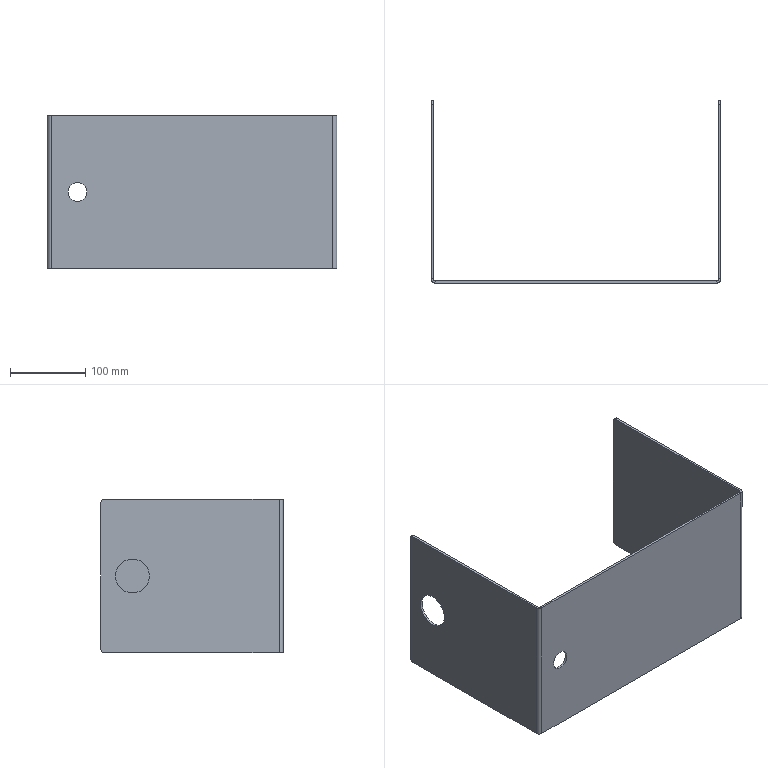Part | SolidWorks | features ICE 2, Fillet 1, FlatPattern 1, SMBaseFlange 1, SheetMetal 1, UnFold 1 | 1 solid | 30 faces | box 384 x 242 x 204 mm | volume 519134 mm3 | plane 18 | cylinder 12 | commonest cylinder face diameters 10 x4 5 x2 11 x2 25 x2 45 x2
STEP:
#1=CARTESIAN_POINT('',(-152.,0.,-12.5));
#2=VERTEX_POINT('',#1);
#3=CARTESIAN_POINT('',(-152.,0.,12.5));
#4=VERTEX_POINT('',#3);
#5=CARTESIAN_POINT('',(-152.,0.,0.));
#6=DIRECTION('',(0.,1.,0.));
#7=DIRECTION('',(0.,0.,1.));
#8=AXIS2_PLACEMENT_3D('',#5,#6,#7);
#9=CIRCLE('',#8,12.5);
#10=EDGE_CURVE('',#2,#4,#9,.T.);
#11=ORIENTED_EDGE('',*,*,#10,.F.);
#12=CARTESIAN_POINT('',(-152.,3.,-12.5));
#13=VERTEX_POINT('',#12);
#14=CARTESIAN_POINT('',(-152.,0.,-12.5));
#15=DIRECTION('',(0.,1.,0.));
#16=VECTOR('',#15,1000.);
#17=LINE('',#14,#16);
#18=EDGE_CURVE('',#2,#13,#17,.T.);
#19=ORIENTED_EDGE('',*,*,#18,.T.);
#20=CARTESIAN_POINT('',(-152.,3.,12.5));
#21=VERTEX_POINT('',#20);
#22=CARTESIAN_POINT('',(-152.,3.,0.));
#23=DIRECTION('',(0.,1.,0.));
#24=DIRECTION('',(0.,0.,1.));
#25=AXIS2_PLACEMENT_3D('',#22,#23,#24);
#26=CIRCLE('',#25,12.5);
#27=EDGE_CURVE('',#13,#21,#26,.T.);
#28=ORIENTED_EDGE('',*,*,#27,.T.);
#29=CARTESIAN_POINT('',(-152.,0.,12.5));
#30=DIRECTION('',(0.,1.,0.));
#31=VECTOR('',#30,1000.);
#32=LINE('',#29,#31);
#33=EDGE_CURVE('',#4,#21,#32,.T.);
#34=ORIENTED_EDGE('',*,*,#33,.F.);
#35=EDGE_LOOP('',(#11,#19,#28,#34));
#36=FACE_OUTER_BOUND('',#35,.T.);
#37=CARTESIAN_POINT('',(-152.,0.,0.));
#38=DIRECTION('',(0.,1.,0.));
#39=DIRECTION('',(0.,0.,1.));
#40=AXIS2_PLACEMENT_3D('',#37,#38,#39);
#41=CYLINDRICAL_SURFACE('',#40,12.5);
#42=ADVANCED_FACE('',(#36),#41,.F.);
#43=CARTESIAN_POINT('',(-189.,200.,-22.5));
#44=VERTEX_POINT('',#43);
#45=CARTESIAN_POINT('',(-189.,200.,22.5));
#46=VERTEX_POINT('',#45);
#47=CARTESIAN_POINT('',(-189.,200.,0.));
#48=DIRECTION('',(-1.,0.,0.));
#49=DIRECTION('',(0.,0.,1.));
#50=AXIS2_PLACEMENT_3D('',#47,#48,#49);
#51=CIRCLE('',#50,22.5);
#52=EDGE_CURVE('',#44,#46,#51,.T.);
#53=ORIENTED_EDGE('',*,*,#52,.F.);
#54=CARTESIAN_POINT('',(-192.,200.,-22.5));
#55=VERTEX_POINT('',#54);
#56=CARTESIAN_POINT('',(-189.,200.,-22.5));
#57=DIRECTION('',(-1.,0.,0.));
#58=VECTOR('',#57,1000.);
#59=LINE('',#56,#58);
#60=EDGE_CURVE('',#44,#55,#59,.T.);
#61=ORIENTED_EDGE('',*,*,#60,.T.);
#62=CARTESIAN_POINT('',(-192.,200.,22.5));
#63=VERTEX_POINT('',#62);
#64=CARTESIAN_POINT('',(-192.,200.,0.));
#65=DIRECTION('',(-1.,0.,0.));
#66=DIRECTION('',(0.,0.,1.));
#67=AXIS2_PLACEMENT_3D('',#64,#65,#66);
#68=CIRCLE('',#67,22.5);
#69=EDGE_CURVE('',#55,#63,#68,.T.);
#70=ORIENTED_EDGE('',*,*,#69,.T.);
#71=CARTESIAN_POINT('',(-189.,200.,22.5));
#72=DIRECTION('',(-1.,0.,0.));
#73=VECTOR('',#72,1000.);
#74=LINE('',#71,#73);
#75=EDGE_CURVE('',#46,#63,#74,.T.);
#76=ORIENTED_EDGE('',*,*,#75,.F.);
#77=EDGE_LOOP('',(#53,#61,#70,#76));
#78=FACE_OUTER_BOUND('',#77,.T.);
#79=CARTESIAN_POINT('',(-189.,200.,0.));
#80=DIRECTION('',(-1.,0.,0.));
#81=DIRECTION('',(0.,0.,1.));
#82=AXIS2_PLACEMENT_3D('',#79,#80,#81);
#83=CYLINDRICAL_SURFACE('',#82,22.5);
#84=ADVANCED_FACE('',(#78),#83,.F.);
#85=CARTESIAN_POINT('',(186.5,0.,102.));
#86=VERTEX_POINT('',#85);
#87=CARTESIAN_POINT('',(186.5,3.,102.));
#88=VERTEX_POINT('',#87);
#89=CARTESIAN_POINT('',(186.5,0.,102.));
#90=DIRECTION('',(0.,1.,0.));
#91=VECTOR('',#90,1000.);
#92=LINE('',#89,#91);
#93=EDGE_CURVE('',#86,#88,#92,.T.);
#94=ORIENTED_EDGE('',*,*,#93,.F.);
#95=CARTESIAN_POINT('',(192.,5.5,102.));
#96=VERTEX_POINT('',#95);
#97=CARTESIAN_POINT('',(186.5,5.5,102.));
#98=DIRECTION('',(0.,0.,-1.));
#99=DIRECTION('',(1.,0.,0.));
#100=AXIS2_PLACEMENT_3D('',#97,#98,#99);
#101=CIRCLE('',#100,5.5);
#102=EDGE_CURVE('',#96,#86,#101,.T.);
#103=ORIENTED_EDGE('',*,*,#102,.F.);
#104=CARTESIAN_POINT('',(189.,5.5,102.));
#105=VERTEX_POINT('',#104);
#106=CARTESIAN_POINT('',(189.,5.5,102.));
#107=DIRECTION('',(1.,0.,0.));
#108=VECTOR('',#107,1000.);
#109=LINE('',#106,#108);
#110=EDGE_CURVE('',#105,#96,#109,.T.);
#111=ORIENTED_EDGE('',*,*,#110,.F.);
#112=CARTESIAN_POINT('',(186.5,5.5,102.));
#113=DIRECTION('',(0.,0.,-1.));
#114=DIRECTION('',(1.,0.,0.));
#115=AXIS2_PLACEMENT_3D('',#112,#113,#114);
#116=CIRCLE('',#115,2.5);
#117=EDGE_CURVE('',#105,#88,#116,.T.);
#118=ORIENTED_EDGE('',*,*,#117,.T.);
#119=EDGE_LOOP('',(#94,#103,#111,#118));
#120=FACE_OUTER_BOUND('',#119,.T.);
#121=CARTESIAN_POINT('',(186.5,0.,102.));
#122=DIRECTION('',(0.,0.,1.));
#123=DIRECTION('',(1.,0.,0.));
#124=AXIS2_PLACEMENT_3D('',#121,#122,#123);
#125=PLANE('',#124);
#126=ADVANCED_FACE('',(#120),#125,.T.);
#127=CARTESIAN_POINT('',(-186.5,0.,102.));
#128=VERTEX_POINT('',#127);
#129=CARTESIAN_POINT('',(-192.,0.,102.));
#130=DIRECTION('',(-1.,0.,0.));
#131=VECTOR('',#130,1000.);
#132=LINE('',#129,#131);
#133=EDGE_CURVE('',#86,#128,#132,.T.);
#134=ORIENTED_EDGE('',*,*,#133,.F.);
#135=ORIENTED_EDGE('',*,*,#93,.T.);
#136=CARTESIAN_POINT('',(-186.5,3.,102.));
#137=VERTEX_POINT('',#136);
#138=CARTESIAN_POINT('',(-192.,3.,102.));
#139=DIRECTION('',(-1.,0.,0.));
#140=VECTOR('',#139,1000.);
#141=LINE('',#138,#140);
#142=EDGE_CURVE('',#88,#137,#141,.T.);
#143=ORIENTED_EDGE('',*,*,#142,.T.);
#144=CARTESIAN_POINT('',(-186.5,3.,102.));
#145=DIRECTION('',(0.,-1.,0.));
#146=VECTOR('',#145,1000.);
#147=LINE('',#144,#146);
#148=EDGE_CURVE('',#137,#128,#147,.T.);
#149=ORIENTED_EDGE('',*,*,#148,.T.);
#150=EDGE_LOOP('',(#134,#135,#143,#149));
#151=FACE_OUTER_BOUND('',#150,.T.);
#152=CARTESIAN_POINT('',(189.,5.5,102.));
#153=DIRECTION('',(0.,0.,1.));
#154=DIRECTION('',(1.,0.,0.));
#155=AXIS2_PLACEMENT_3D('',#152,#153,#154);
#156=PLANE('',#155);
#157=ADVANCED_FACE('',(#151),#156,.T.);
#158=CARTESIAN_POINT('',(192.,5.5,-102.));
#159=VERTEX_POINT('',#158);
#160=CARTESIAN_POINT('',(189.,5.5,-102.));
#161=VERTEX_POINT('',#160);
#162=CARTESIAN_POINT('',(192.,5.5,-102.));
#163=DIRECTION('',(-1.,0.,0.));
#164=VECTOR('',#163,1000.);
#165=LINE('',#162,#164);
#166=EDGE_CURVE('',#159,#161,#165,.T.);
#167=ORIENTED_EDGE('',*,*,#166,.F.);
#168=CARTESIAN_POINT('',(186.5,0.,-102.));
#169=VERTEX_POINT('',#168);
#170=CARTESIAN_POINT('',(186.5,5.5,-102.));
#171=DIRECTION('',(0.,0.,-1.));
#172=DIRECTION('',(1.,0.,0.));
#173=AXIS2_PLACEMENT_3D('',#170,#171,#172);
#174=CIRCLE('',#173,5.5);
#175=EDGE_CURVE('',#159,#169,#174,.T.);
#176=ORIENTED_EDGE('',*,*,#175,.T.);
#177=CARTESIAN_POINT('',(186.5,3.,-102.));
#178=VERTEX_POINT('',#177);
#179=CARTESIAN_POINT('',(186.5,3.,-102.));
#180=DIRECTION('',(0.,-1.,0.));
#181=VECTOR('',#180,1000.);
#182=LINE('',#179,#181);
#183=EDGE_CURVE('',#178,#169,#182,.T.);
#184=ORIENTED_EDGE('',*,*,#183,.F.);
#185=CARTESIAN_POINT('',(186.5,5.5,-102.));
#186=DIRECTION('',(0.,0.,-1.));
#187=DIRECTION('',(1.,0.,0.));
#188=AXIS2_PLACEMENT_3D('',#185,#186,#187);
#189=CIRCLE('',#188,2.5);
#190=EDGE_CURVE('',#161,#178,#189,.T.);
#191=ORIENTED_EDGE('',*,*,#190,.F.);
#192=EDGE_LOOP('',(#167,#176,#184,#191));
#193=FACE_OUTER_BOUND('',#192,.T.);
#194=CARTESIAN_POINT('',(192.,5.5,-102.));
#195=DIRECTION('',(0.,0.,-1.));
#196=DIRECTION('',(-1.,0.,0.));
#197=AXIS2_PLACEMENT_3D('',#194,#195,#196);
#198=PLANE('',#197);
#199=ADVANCED_FACE('',(#193),#198,.T.);
#200=CARTESIAN_POINT('',(189.,237.,-102.));
#201=VERTEX_POINT('',#200);
#202=CARTESIAN_POINT('',(189.,0.,-102.));
#203=DIRECTION('',(0.,-1.,0.));
#204=VECTOR('',#203,1000.);
#205=LINE('',#202,#204);
#206=EDGE_CURVE('',#201,#161,#205,.T.);
#207=ORIENTED_EDGE('',*,*,#206,.F.);
#208=CARTESIAN_POINT('',(192.,237.,-102.));
#209=VERTEX_POINT('',#208);
#210=CARTESIAN_POINT('',(186.5,237.,-102.));
#211=DIRECTION('',(1.,0.,0.));
#212=VECTOR('',#211,1000.);
#213=LINE('',#210,#212);
#214=EDGE_CURVE('',#201,#209,#213,.T.);
#215=ORIENTED_EDGE('',*,*,#214,.T.);
#216=CARTESIAN_POINT('',(192.,0.,-102.));
#217=DIRECTION('',(0.,-1.,0.));
#218=VECTOR('',#217,1000.);
#219=LINE('',#216,#218);
#220=EDGE_CURVE('',#209,#159,#219,.T.);
#221=ORIENTED_EDGE('',*,*,#220,.T.);
#222=ORIENTED_EDGE('',*,*,#166,.T.);
#223=EDGE_LOOP('',(#207,#215,#221,#222));
#224=FACE_OUTER_BOUND('',#223,.T.);
#225=CARTESIAN_POINT('',(186.5,3.,-102.));
#226=DIRECTION('',(0.,0.,-1.));
#227=DIRECTION('',(-1.,0.,0.));
#228=AXIS2_PLACEMENT_3D('',#225,#226,#227);
#229=PLANE('',#228);
#230=ADVANCED_FACE('',(#224),#229,.T.);
#231=CARTESIAN_POINT('',(-192.,5.5,102.));
#232=VERTEX_POINT('',#231);
#233=CARTESIAN_POINT('',(-189.,5.5,102.));
#234=VERTEX_POINT('',#233);
#235=CARTESIAN_POINT('',(-192.,5.5,102.));
#236=DIRECTION('',(1.,0.,0.));
#237=VECTOR('',#236,1000.);
#238=LINE('',#235,#237);
#239=EDGE_CURVE('',#232,#234,#238,.T.);
#240=ORIENTED_EDGE('',*,*,#239,.F.);
#241=CARTESIAN_POINT('',(-186.5,5.5,102.));
#242=DIRECTION('',(0.,0.,-1.));
#243=DIRECTION('',(1.,0.,0.));
#244=AXIS2_PLACEMENT_3D('',#241,#242,#243);
#245=CIRCLE('',#244,5.5);
#246=EDGE_CURVE('',#128,#232,#245,.T.);
#247=ORIENTED_EDGE('',*,*,#246,.F.);
#248=ORIENTED_EDGE('',*,*,#148,.F.);
#249=CARTESIAN_POINT('',(-186.5,5.5,102.));
#250=DIRECTION('',(0.,0.,-1.));
#251=DIRECTION('',(1.,0.,0.));
#252=AXIS2_PLACEMENT_3D('',#249,#250,#251);
#253=CIRCLE('',#252,2.5);
#254=EDGE_CURVE('',#137,#234,#253,.T.);
#255=ORIENTED_EDGE('',*,*,#254,.T.);
#256=EDGE_LOOP('',(#240,#247,#248,#255));
#257=FACE_OUTER_BOUND('',#256,.T.);
#258=CARTESIAN_POINT('',(-192.,5.5,102.));
#259=DIRECTION('',(0.,0.,1.));
#260=DIRECTION('',(1.,0.,0.));
#261=AXIS2_PLACEMENT_3D('',#258,#259,#260);
#262=PLANE('',#261);
#263=ADVANCED_FACE('',(#257),#262,.T.);
#264=CARTESIAN_POINT('',(-189.,237.,102.));
#265=VERTEX_POINT('',#264);
#266=CARTESIAN_POINT('',(-189.,0.,102.));
#267=DIRECTION('',(0.,1.,0.));
#268=VECTOR('',#267,1000.);
#269=LINE('',#266,#268);
#270=EDGE_CURVE('',#234,#265,#269,.T.);
#271=ORIENTED_EDGE('',*,*,#270,.T.);
#272=CARTESIAN_POINT('',(-192.,237.,102.));
#273=VERTEX_POINT('',#272);
#274=CARTESIAN_POINT('',(-186.5,237.,102.));
#275=DIRECTION('',(-1.,0.,0.));
#276=VECTOR('',#275,1000.);
#277=LINE('',#274,#276);
#278=EDGE_CURVE('',#265,#273,#277,.T.);
#279=ORIENTED_EDGE('',*,*,#278,.T.);
#280=CARTESIAN_POINT('',(-192.,0.,102.));
#281=DIRECTION('',(0.,1.,0.));
#282=VECTOR('',#281,1000.);
#283=LINE('',#280,#282);
#284=EDGE_CURVE('',#232,#273,#283,.T.);
#285=ORIENTED_EDGE('',*,*,#284,.F.);
#286=ORIENTED_EDGE('',*,*,#239,.T.);
#287=EDGE_LOOP('',(#271,#279,#285,#286));
#288=FACE_OUTER_BOUND('',#287,.T.);
#289=CARTESIAN_POINT('',(-186.5,3.,102.));
#290=DIRECTION('',(0.,0.,1.));
#291=DIRECTION('',(1.,0.,0.));
#292=AXIS2_PLACEMENT_3D('',#289,#290,#291);
#293=PLANE('',#292);
#294=ADVANCED_FACE('',(#288),#293,.T.);
#295=CARTESIAN_POINT('',(-186.5,0.,-102.));
#296=VERTEX_POINT('',#295);
#297=CARTESIAN_POINT('',(-186.5,3.,-102.));
#298=VERTEX_POINT('',#297);
#299=CARTESIAN_POINT('',(-186.5,0.,-102.));
#300=DIRECTION('',(0.,1.,0.));
#301=VECTOR('',#300,1000.);
#302=LINE('',#299,#301);
#303=EDGE_CURVE('',#296,#298,#302,.T.);
#304=ORIENTED_EDGE('',*,*,#303,.F.);
#305=CARTESIAN_POINT('',(-192.,5.5,-102.));
#306=VERTEX_POINT('',#305);
#307=CARTESIAN_POINT('',(-186.5,5.5,-102.));
#308=DIRECTION('',(0.,0.,-1.));
#309=DIRECTION('',(1.,0.,0.));
#310=AXIS2_PLACEMENT_3D('',#307,#308,#309);
#311=CIRCLE('',#310,5.5);
#312=EDGE_CURVE('',#296,#306,#311,.T.);
#313=ORIENTED_EDGE('',*,*,#312,.T.);
#314=CARTESIAN_POINT('',(-189.,5.5,-102.));
#315=VERTEX_POINT('',#314);
#316=CARTESIAN_POINT('',(-189.,5.5,-102.));
#317=DIRECTION('',(-1.,0.,0.));
#318=VECTOR('',#317,1000.);
#319=LINE('',#316,#318);
#320=EDGE_CURVE('',#315,#306,#319,.T.);
#321=ORIENTED_EDGE('',*,*,#320,.F.);
#322=CARTESIAN_POINT('',(-186.5,5.5,-102.));
#323=DIRECTION('',(0.,0.,-1.));
#324=DIRECTION('',(1.,0.,0.));
#325=AXIS2_PLACEMENT_3D('',#322,#323,#324);
#326=CIRCLE('',#325,2.5);
#327=EDGE_CURVE('',#298,#315,#326,.T.);
#328=ORIENTED_EDGE('',*,*,#327,.F.);
#329=EDGE_LOOP('',(#304,#313,#321,#328));
#330=FACE_OUTER_BOUND('',#329,.T.);
#331=CARTESIAN_POINT('',(-186.5,0.,-102.));
#332=DIRECTION('',(0.,0.,-1.));
#333=DIRECTION('',(-1.,0.,0.));
#334=AXIS2_PLACEMENT_3D('',#331,#332,#333);
#335=PLANE('',#334);
#336=ADVANCED_FACE('',(#330),#335,.T.);
#337=CARTESIAN_POINT('',(-192.,0.,-102.));
#338=DIRECTION('',(-1.,0.,0.));
#339=VECTOR('',#338,1000.);
#340=LINE('',#337,#339);
#341=EDGE_CURVE('',#169,#296,#340,.T.);
#342=ORIENTED_EDGE('',*,*,#341,.T.);
#343=ORIENTED_EDGE('',*,*,#303,.T.);
#344=CARTESIAN_POINT('',(-192.,3.,-102.));
#345=DIRECTION('',(-1.,0.,0.));
#346=VECTOR('',#345,1000.);
#347=LINE('',#344,#346);
#348=EDGE_CURVE('',#178,#298,#347,.T.);
#349=ORIENTED_EDGE('',*,*,#348,.F.);
#350=ORIENTED_EDGE('',*,*,#183,.T.);
#351=EDGE_LOOP('',(#342,#343,#349,#350));
#352=FACE_OUTER_BOUND('',#351,.T.);
#353=CARTESIAN_POINT('',(-189.,5.5,-102.));
#354=DIRECTION('',(0.,0.,-1.));
#355=DIRECTION('',(-1.,0.,0.));
#356=AXIS2_PLACEMENT_3D('',#353,#354,#355);
#357=PLANE('',#356);
#358=ADVANCED_FACE('',(#352),#357,.T.);
#359=CARTESIAN_POINT('',(-189.,200.,0.));
#360=DIRECTION('',(-1.,0.,0.));
#361=DIRECTION('',(0.,0.,1.));
#362=AXIS2_PLACEMENT_3D('',#359,#360,#361);
#363=CIRCLE('',#362,22.5);
#364=EDGE_CURVE('',#46,#44,#363,.T.);
#365=ORIENTED_EDGE('',*,*,#364,.T.);
#366=ORIENTED_EDGE('',*,*,#52,.T.);
#367=EDGE_LOOP('',(#365,#366));
#368=FACE_BOUND('',#367,.T.);
#369=CARTESIAN_POINT('',(-189.,242.,97.));
#370=VERTEX_POINT('',#369);
#371=CARTESIAN_POINT('',(-189.,242.,-97.));
#372=VERTEX_POINT('',#371);
#373=CARTESIAN_POINT('',(-189.,242.,102.));
#374=DIRECTION('',(0.,0.,-1.));
#375=VECTOR('',#374,1000.);
#376=LINE('',#373,#375);
#377=EDGE_CURVE('',#370,#372,#376,.T.);
#378=ORIENTED_EDGE('',*,*,#377,.F.);
#379=CARTESIAN_POINT('',(-189.,237.,97.));
#380=DIRECTION('',(1.,0.,0.));
#381=DIRECTION('',(0.,0.,1.));
#382=AXIS2_PLACEMENT_3D('',#379,#380,#381);
#383=CIRCLE('',#382,5.);
#384=EDGE_CURVE('',#370,#265,#383,.T.);
#385=ORIENTED_EDGE('',*,*,#384,.T.);
#386=ORIENTED_EDGE('',*,*,#270,.F.);
#387=CARTESIAN_POINT('',(-189.,5.5,102.));
#388=DIRECTION('',(0.,0.,-1.));
#389=VECTOR('',#388,1000.);
#390=LINE('',#387,#389);
#391=EDGE_CURVE('',#234,#315,#390,.T.);
#392=ORIENTED_EDGE('',*,*,#391,.T.);
#393=CARTESIAN_POINT('',(-189.,237.,-102.));
#394=VERTEX_POINT('',#393);
#395=CARTESIAN_POINT('',(-189.,0.,-102.));
#396=DIRECTION('',(0.,1.,0.));
#397=VECTOR('',#396,1000.);
#398=LINE('',#395,#397);
#399=EDGE_CURVE('',#315,#394,#398,.T.);
#400=ORIENTED_EDGE('',*,*,#399,.T.);
#401=CARTESIAN_POINT('',(-189.,237.,-97.));
#402=DIRECTION('',(1.,0.,0.));
#403=DIRECTION('',(0.,0.,1.));
#404=AXIS2_PLACEMENT_3D('',#401,#402,#403);
#405=CIRCLE('',#404,5.);
#406=EDGE_CURVE('',#394,#372,#405,.T.);
#407=ORIENTED_EDGE('',*,*,#406,.T.);
#408=EDGE_LOOP('',(#378,#385,#386,#392,#400,#407));
#409=FACE_OUTER_BOUND('',#408,.T.);
#410=CARTESIAN_POINT('',(-189.,0.,102.));
#411=DIRECTION('',(-1.,0.,0.));
#412=DIRECTION('',(0.,0.,1.));
#413=AXIS2_PLACEMENT_3D('',#410,#411,#412);
#414=PLANE('',#413);
#415=ADVANCED_FACE('',(#368,#409),#414,.F.);
#416=CARTESIAN_POINT('',(-192.,242.,97.));
#417=VERTEX_POINT('',#416);
#418=CARTESIAN_POINT('',(-192.,242.,-97.));
#419=VERTEX_POINT('',#418);
#420=CARTESIAN_POINT('',(-192.,242.,102.));
#421=DIRECTION('',(0.,0.,-1.));
#422=VECTOR('',#421,1000.);
#423=LINE('',#420,#422);
#424=EDGE_CURVE('',#417,#419,#423,.T.);
#425=ORIENTED_EDGE('',*,*,#424,.F.);
#426=CARTESIAN_POINT('',(-192.,242.,97.));
#427=DIRECTION('',(1.,0.,0.));
#428=VECTOR('',#427,1000.);
#429=LINE('',#426,#428);
#430=EDGE_CURVE('',#417,#370,#429,.T.);
#431=ORIENTED_EDGE('',*,*,#430,.T.);
#432=ORIENTED_EDGE('',*,*,#377,.T.);
#433=CARTESIAN_POINT('',(-192.,242.,-97.));
#434=DIRECTION('',(-1.,0.,0.));
#435=VECTOR('',#434,1000.);
#436=LINE('',#433,#435);
#437=EDGE_CURVE('',#372,#419,#436,.T.);
#438=ORIENTED_EDGE('',*,*,#437,.T.);
#439=EDGE_LOOP('',(#425,#431,#432,#438));
#440=FACE_OUTER_BOUND('',#439,.T.);
#441=CARTESIAN_POINT('',(-192.,242.,102.));
#442=DIRECTION('',(0.,1.,0.));
#443=DIRECTION('',(0.,0.,1.));
#444=AXIS2_PLACEMENT_3D('',#441,#442,#443);
#445=PLANE('',#444);
#446=ADVANCED_FACE('',(#440),#445,.T.);
#447=CARTESIAN_POINT('',(-192.,200.,0.));
#448=DIRECTION('',(-1.,0.,0.));
#449=DIRECTION('',(0.,0.,1.));
#450=AXIS2_PLACEMENT_3D('',#447,#448,#449);
#451=CIRCLE('',#450,22.5);
#452=EDGE_CURVE('',#63,#55,#451,.T.);
#453=ORIENTED_EDGE('',*,*,#452,.F.);
#454=ORIENTED_EDGE('',*,*,#69,.F.);
#455=EDGE_LOOP('',(#453,#454));
#456=FACE_BOUND('',#455,.T.);
#457=ORIENTED_EDGE('',*,*,#284,.T.);
#458=CARTESIAN_POINT('',(-192.,237.,97.));
#459=DIRECTION('',(-1.,0.,0.));
#460=DIRECTION('',(0.,0.,1.));
#461=AXIS2_PLACEMENT_3D('',#458,#459,#460);
#462=CIRCLE('',#461,5.);
#463=EDGE_CURVE('',#273,#417,#462,.T.);
#464=ORIENTED_EDGE('',*,*,#463,.T.);
#465=ORIENTED_EDGE('',*,*,#424,.T.);
#466=CARTESIAN_POINT('',(-192.,237.,-102.));
#467=VERTEX_POINT('',#466);
#468=CARTESIAN_POINT('',(-192.,237.,-97.));
#469=DIRECTION('',(-1.,0.,0.));
#470=DIRECTION('',(0.,0.,1.));
#471=AXIS2_PLACEMENT_3D('',#468,#469,#470);
#472=CIRCLE('',#471,5.);
#473=EDGE_CURVE('',#419,#467,#472,.T.);
#474=ORIENTED_EDGE('',*,*,#473,.T.);
#475=CARTESIAN_POINT('',(-192.,0.,-102.));
#476=DIRECTION('',(0.,1.,0.));
#477=VECTOR('',#476,1000.);
#478=LINE('',#475,#477);
#479=EDGE_CURVE('',#306,#467,#478,.T.);
#480=ORIENTED_EDGE('',*,*,#479,.F.);
#481=CARTESIAN_POINT('',(-192.,5.5,102.));
#482=DIRECTION('',(0.,0.,-1.));
#483=VECTOR('',#482,1000.);
#484=LINE('',#481,#483);
#485=EDGE_CURVE('',#232,#306,#484,.T.);
#486=ORIENTED_EDGE('',*,*,#485,.F.);
#487=EDGE_LOOP('',(#457,#464,#465,#474,#480,#486));
#488=FACE_OUTER_BOUND('',#487,.T.);
#489=CARTESIAN_POINT('',(-192.,0.,102.));
#490=DIRECTION('',(-1.,0.,0.));
#491=DIRECTION('',(0.,0.,1.));
#492=AXIS2_PLACEMENT_3D('',#489,#490,#491);
#493=PLANE('',#492);
#494=ADVANCED_FACE('',(#456,#488),#493,.T.);
#495=ORIENTED_EDGE('',*,*,#312,.F.);
#496=CARTESIAN_POINT('',(-186.5,0.,102.));
#497=DIRECTION('',(0.,0.,-1.));
#498=VECTOR('',#497,1000.);
#499=LINE('',#496,#498);
#500=EDGE_CURVE('',#128,#296,#499,.T.);
#501=ORIENTED_EDGE('',*,*,#500,.F.);
#502=ORIENTED_EDGE('',*,*,#246,.T.);
#503=ORIENTED_EDGE('',*,*,#485,.T.);
#504=EDGE_LOOP('',(#495,#501,#502,#503));
#505=FACE_OUTER_BOUND('',#504,.T.);
#506=CARTESIAN_POINT('',(-186.5,5.5,102.));
#507=DIRECTION('',(0.,0.,-1.));
#508=DIRECTION('',(-1.,0.,0.));
#509=AXIS2_PLACEMENT_3D('',#506,#507,#508);
#510=CYLINDRICAL_SURFACE('',#509,5.5);
#511=ADVANCED_FACE('',(#505),#510,.T.);
#512=CARTESIAN_POINT('',(-152.,0.,0.));
#513=DIRECTION('',(0.,1.,0.));
#514=DIRECTION('',(0.,0.,1.));
#515=AXIS2_PLACEMENT_3D('',#512,#513,#514);
#516=CIRCLE('',#515,12.5);
#517=EDGE_CURVE('',#4,#2,#516,.T.);
#518=ORIENTED_EDGE('',*,*,#517,.T.);
#519=ORIENTED_EDGE('',*,*,#10,.T.);
#520=EDGE_LOOP('',(#518,#519));
#521=FACE_BOUND('',#520,.T.);
#522=ORIENTED_EDGE('',*,*,#341,.F.);
#523=CARTESIAN_POINT('',(186.5,0.,102.));
#524=DIRECTION('',(0.,0.,-1.));
#525=VECTOR('',#524,1000.);
#526=LINE('',#523,#525);
#527=EDGE_CURVE('',#86,#169,#526,.T.);
#528=ORIENTED_EDGE('',*,*,#527,.F.);
#529=ORIENTED_EDGE('',*,*,#133,.T.);
#530=ORIENTED_EDGE('',*,*,#500,.T.);
#531=EDGE_LOOP('',(#522,#528,#529,#530));
#532=FACE_OUTER_BOUND('',#531,.T.);
#533=CARTESIAN_POINT('',(-192.,0.,102.));
#534=DIRECTION('',(0.,-1.,0.));
#535=DIRECTION('',(0.,0.,-1.));
#536=AXIS2_PLACEMENT_3D('',#533,#534,#535);
#537=PLANE('',#536);
#538=ADVANCED_FACE('',(#521,#532),#537,.T.);
#539=ORIENTED_EDGE('',*,*,#175,.F.);
#540=CARTESIAN_POINT('',(192.,5.5,102.));
#541=DIRECTION('',(0.,0.,-1.));
#542=VECTOR('',#541,1000.);
#543=LINE('',#540,#542);
#544=EDGE_CURVE('',#96,#159,#543,.T.);
#545=ORIENTED_EDGE('',*,*,#544,.F.);
#546=ORIENTED_EDGE('',*,*,#102,.T.);
#547=ORIENTED_EDGE('',*,*,#527,.T.);
#548=EDGE_LOOP('',(#539,#545,#546,#547));
#549=FACE_OUTER_BOUND('',#548,.T.);
#550=CARTESIAN_POINT('',(186.5,5.5,102.));
#551=DIRECTION('',(0.,0.,-1.));
#552=DIRECTION('',(-1.,0.,0.));
#553=AXIS2_PLACEMENT_3D('',#550,#551,#552);
#554=CYLINDRICAL_SURFACE('',#553,5.5);
#555=ADVANCED_FACE('',(#549),#554,.T.);
#556=CARTESIAN_POINT('',(192.,242.,97.));
#557=VERTEX_POINT('',#556);
#558=CARTESIAN_POINT('',(192.,242.,-97.));
#559=VERTEX_POINT('',#558);
#560=CARTESIAN_POINT('',(192.,242.,102.));
#561=DIRECTION('',(0.,0.,-1.));
#562=VECTOR('',#561,1000.);
#563=LINE('',#560,#562);
#564=EDGE_CURVE('',#557,#559,#563,.T.);
#565=ORIENTED_EDGE('',*,*,#564,.F.);
#566=CARTESIAN_POINT('',(192.,237.,102.));
#567=VERTEX_POINT('',#566);
#568=CARTESIAN_POINT('',(192.,237.,97.));
#569=DIRECTION('',(1.,0.,0.));
#570=DIRECTION('',(0.,0.,-1.));
#571=AXIS2_PLACEMENT_3D('',#568,#569,#570);
#572=CIRCLE('',#571,5.);
#573=EDGE_CURVE('',#557,#567,#572,.T.);
#574=ORIENTED_EDGE('',*,*,#573,.T.);
#575=CARTESIAN_POINT('',(192.,0.,102.));
#576=DIRECTION('',(0.,-1.,0.));
#577=VECTOR('',#576,1000.);
#578=LINE('',#575,#577);
#579=EDGE_CURVE('',#567,#96,#578,.T.);
#580=ORIENTED_EDGE('',*,*,#579,.T.);
#581=ORIENTED_EDGE('',*,*,#544,.T.);
#582=ORIENTED_EDGE('',*,*,#220,.F.);
#583=CARTESIAN_POINT('',(192.,237.,-97.));
#584=DIRECTION('',(1.,0.,0.));
#585=DIRECTION('',(0.,0.,-1.));
#586=AXIS2_PLACEMENT_3D('',#583,#584,#585);
#587=CIRCLE('',#586,5.);
#588=EDGE_CURVE('',#209,#559,#587,.T.);
#589=ORIENTED_EDGE('',*,*,#588,.T.);
#590=EDGE_LOOP('',(#565,#574,#580,#581,#582,#589));
#591=FACE_OUTER_BOUND('',#590,.T.);
#592=CARTESIAN_POINT('',(192.,0.,102.));
#593=DIRECTION('',(1.,0.,0.));
#594=DIRECTION('',(0.,0.,-1.));
#595=AXIS2_PLACEMENT_3D('',#592,#593,#594);
#596=PLANE('',#595);
#597=ADVANCED_FACE('',(#591),#596,.T.);
#598=CARTESIAN_POINT('',(189.,242.,97.));
#599=VERTEX_POINT('',#598);
#600=CARTESIAN_POINT('',(189.,242.,-97.));
#601=VERTEX_POINT('',#600);
#602=CARTESIAN_POINT('',(189.,242.,102.));
#603=DIRECTION('',(0.,0.,-1.));
#604=VECTOR('',#603,1000.);
#605=LINE('',#602,#604);
#606=EDGE_CURVE('',#599,#601,#605,.T.);
#607=ORIENTED_EDGE('',*,*,#606,.F.);
#608=CARTESIAN_POINT('',(189.,242.,97.));
#609=DIRECTION('',(1.,0.,0.));
#610=VECTOR('',#609,1000.);
#611=LINE('',#608,#610);
#612=EDGE_CURVE('',#599,#557,#611,.T.);
#613=ORIENTED_EDGE('',*,*,#612,.T.);
#614=ORIENTED_EDGE('',*,*,#564,.T.);
#615=CARTESIAN_POINT('',(189.,242.,-97.));
#616=DIRECTION('',(-1.,0.,0.));
#617=VECTOR('',#616,1000.);
#618=LINE('',#615,#617);
#619=EDGE_CURVE('',#559,#601,#618,.T.);
#620=ORIENTED_EDGE('',*,*,#619,.T.);
#621=EDGE_LOOP('',(#607,#613,#614,#620));
#622=FACE_OUTER_BOUND('',#621,.T.);
#623=CARTESIAN_POINT('',(189.,242.,102.));
#624=DIRECTION('',(0.,1.,0.));
#625=DIRECTION('',(0.,0.,1.));
#626=AXIS2_PLACEMENT_3D('',#623,#624,#625);
#627=PLANE('',#626);
#628=ADVANCED_FACE('',(#622),#627,.T.);
#629=CARTESIAN_POINT('',(189.,237.,102.));
#630=VERTEX_POINT('',#629);
#631=CARTESIAN_POINT('',(189.,0.,102.));
#632=DIRECTION('',(0.,-1.,0.));
#633=VECTOR('',#632,1000.);
#634=LINE('',#631,#633);
#635=EDGE_CURVE('',#630,#105,#634,.T.);
#636=ORIENTED_EDGE('',*,*,#635,.F.);
#637=CARTESIAN_POINT('',(189.,237.,97.));
#638=DIRECTION('',(-1.,0.,0.));
#639=DIRECTION('',(0.,0.,-1.));
#640=AXIS2_PLACEMENT_3D('',#637,#638,#639);
#641=CIRCLE('',#640,5.);
#642=EDGE_CURVE('',#630,#599,#641,.T.);
#643=ORIENTED_EDGE('',*,*,#642,.T.);
#644=ORIENTED_EDGE('',*,*,#606,.T.);
#645=CARTESIAN_POINT('',(189.,237.,-97.));
#646=DIRECTION('',(-1.,0.,0.));
#647=DIRECTION('',(0.,0.,-1.));
#648=AXIS2_PLACEMENT_3D('',#645,#646,#647);
#649=CIRCLE('',#648,5.);
#650=EDGE_CURVE('',#601,#201,#649,.T.);
#651=ORIENTED_EDGE('',*,*,#650,.T.);
#652=ORIENTED_EDGE('',*,*,#206,.T.);
#653=CARTESIAN_POINT('',(189.,5.5,102.));
#654=DIRECTION('',(0.,0.,-1.));
#655=VECTOR('',#654,1000.);
#656=LINE('',#653,#655);
#657=EDGE_CURVE('',#105,#161,#656,.T.);
#658=ORIENTED_EDGE('',*,*,#657,.F.);
#659=EDGE_LOOP('',(#636,#643,#644,#651,#652,#658));
#660=FACE_OUTER_BOUND('',#659,.T.);
#661=CARTESIAN_POINT('',(189.,0.,102.));
#662=DIRECTION('',(1.,0.,0.));
#663=DIRECTION('',(0.,0.,-1.));
#664=AXIS2_PLACEMENT_3D('',#661,#662,#663);
#665=PLANE('',#664);
#666=ADVANCED_FACE('',(#660),#665,.F.);
#667=ORIENTED_EDGE('',*,*,#190,.T.);
#668=CARTESIAN_POINT('',(186.5,3.,102.));
#669=DIRECTION('',(0.,0.,-1.));
#670=VECTOR('',#669,1000.);
#671=LINE('',#668,#670);
#672=EDGE_CURVE('',#88,#178,#671,.T.);
#673=ORIENTED_EDGE('',*,*,#672,.F.);
#674=ORIENTED_EDGE('',*,*,#117,.F.);
#675=ORIENTED_EDGE('',*,*,#657,.T.);
#676=EDGE_LOOP('',(#667,#673,#674,#675));
#677=FACE_OUTER_BOUND('',#676,.T.);
#678=CARTESIAN_POINT('',(186.5,5.5,102.));
#679=DIRECTION('',(0.,0.,-1.));
#680=DIRECTION('',(-1.,0.,0.));
#681=AXIS2_PLACEMENT_3D('',#678,#679,#680);
#682=CYLINDRICAL_SURFACE('',#681,2.5);
#683=ADVANCED_FACE('',(#677),#682,.F.);
#684=CARTESIAN_POINT('',(-152.,3.,0.));
#685=DIRECTION('',(0.,1.,0.));
#686=DIRECTION('',(0.,0.,1.));
#687=AXIS2_PLACEMENT_3D('',#684,#685,#686);
#688=CIRCLE('',#687,12.5);
#689=EDGE_CURVE('',#21,#13,#688,.T.);
#690=ORIENTED_EDGE('',*,*,#689,.F.);
#691=ORIENTED_EDGE('',*,*,#27,.F.);
#692=EDGE_LOOP('',(#690,#691));
#693=FACE_BOUND('',#692,.T.);
#694=ORIENTED_EDGE('',*,*,#348,.T.);
#695=CARTESIAN_POINT('',(-186.5,3.,102.));
#696=DIRECTION('',(0.,0.,-1.));
#697=VECTOR('',#696,1000.);
#698=LINE('',#695,#697);
#699=EDGE_CURVE('',#137,#298,#698,.T.);
#700=ORIENTED_EDGE('',*,*,#699,.F.);
#701=ORIENTED_EDGE('',*,*,#142,.F.);
#702=ORIENTED_EDGE('',*,*,#672,.T.);
#703=EDGE_LOOP('',(#694,#700,#701,#702));
#704=FACE_OUTER_BOUND('',#703,.T.);
#705=CARTESIAN_POINT('',(-192.,3.,102.));
#706=DIRECTION('',(0.,-1.,0.));
#707=DIRECTION('',(0.,0.,-1.));
#708=AXIS2_PLACEMENT_3D('',#705,#706,#707);
#709=PLANE('',#708);
#710=ADVANCED_FACE('',(#693,#704),#709,.F.);
#711=ORIENTED_EDGE('',*,*,#327,.T.);
#712=ORIENTED_EDGE('',*,*,#391,.F.);
#713=ORIENTED_EDGE('',*,*,#254,.F.);
#714=ORIENTED_EDGE('',*,*,#699,.T.);
#715=EDGE_LOOP('',(#711,#712,#713,#714));
#716=FACE_OUTER_BOUND('',#715,.T.);
#717=CARTESIAN_POINT('',(-186.5,5.5,102.));
#718=DIRECTION('',(0.,0.,-1.));
#719=DIRECTION('',(-1.,0.,0.));
#720=AXIS2_PLACEMENT_3D('',#717,#718,#719);
#721=CYLINDRICAL_SURFACE('',#720,2.5);
#722=ADVANCED_FACE('',(#716),#721,.F.);
#723=ORIENTED_EDGE('',*,*,#579,.F.);
#724=CARTESIAN_POINT('',(-186.5,237.,102.));
#725=DIRECTION('',(-1.,0.,0.));
#726=VECTOR('',#725,1000.);
#727=LINE('',#724,#726);
#728=EDGE_CURVE('',#567,#630,#727,.T.);
#729=ORIENTED_EDGE('',*,*,#728,.T.);
#730=ORIENTED_EDGE('',*,*,#635,.T.);
#731=ORIENTED_EDGE('',*,*,#110,.T.);
#732=EDGE_LOOP('',(#723,#729,#730,#731));
#733=FACE_OUTER_BOUND('',#732,.T.);
#734=CARTESIAN_POINT('',(-186.5,5.5,102.));
#735=DIRECTION('',(0.,0.,1.));
#736=DIRECTION('',(1.,0.,0.));
#737=AXIS2_PLACEMENT_3D('',#734,#735,#736);
#738=PLANE('',#737);
#739=ADVANCED_FACE('',(#733),#738,.T.);
#740=ORIENTED_EDGE('',*,*,#479,.T.);
#741=CARTESIAN_POINT('',(-189.,237.,-102.));
#742=DIRECTION('',(1.,0.,0.));
#743=VECTOR('',#742,1000.);
#744=LINE('',#741,#743);
#745=EDGE_CURVE('',#467,#394,#744,.T.);
#746=ORIENTED_EDGE('',*,*,#745,.T.);
#747=ORIENTED_EDGE('',*,*,#399,.F.);
#748=ORIENTED_EDGE('',*,*,#320,.T.);
#749=EDGE_LOOP('',(#740,#746,#747,#748));
#750=FACE_OUTER_BOUND('',#749,.T.);
#751=CARTESIAN_POINT('',(-186.5,5.5,-102.));
#752=DIRECTION('',(0.,0.,1.));
#753=DIRECTION('',(1.,0.,0.));
#754=AXIS2_PLACEMENT_3D('',#751,#752,#753);
#755=PLANE('',#754);
#756=ADVANCED_FACE('',(#750),#755,.F.);
#757=ORIENTED_EDGE('',*,*,#60,.F.);
#758=ORIENTED_EDGE('',*,*,#364,.F.);
#759=ORIENTED_EDGE('',*,*,#75,.T.);
#760=ORIENTED_EDGE('',*,*,#452,.T.);
#761=EDGE_LOOP('',(#757,#758,#759,#760));
#762=FACE_OUTER_BOUND('',#761,.T.);
#763=CARTESIAN_POINT('',(-189.,200.,0.));
#764=DIRECTION('',(-1.,0.,0.));
#765=DIRECTION('',(0.,0.,1.));
#766=AXIS2_PLACEMENT_3D('',#763,#764,#765);
#767=CYLINDRICAL_SURFACE('',#766,22.5);
#768=ADVANCED_FACE('',(#762),#767,.F.);
#769=ORIENTED_EDGE('',*,*,#18,.F.);
#770=ORIENTED_EDGE('',*,*,#517,.F.);
#771=ORIENTED_EDGE('',*,*,#33,.T.);
#772=ORIENTED_EDGE('',*,*,#689,.T.);
#773=EDGE_LOOP('',(#769,#770,#771,#772));
#774=FACE_OUTER_BOUND('',#773,.T.);
#775=CARTESIAN_POINT('',(-152.,0.,0.));
#776=DIRECTION('',(0.,1.,0.));
#777=DIRECTION('',(0.,0.,1.));
#778=AXIS2_PLACEMENT_3D('',#775,#776,#777);
#779=CYLINDRICAL_SURFACE('',#778,12.5);
#780=ADVANCED_FACE('',(#774),#779,.F.);
#781=ORIENTED_EDGE('',*,*,#642,.F.);
#782=ORIENTED_EDGE('',*,*,#728,.F.);
#783=ORIENTED_EDGE('',*,*,#573,.F.);
#784=ORIENTED_EDGE('',*,*,#612,.F.);
#785=EDGE_LOOP('',(#781,#782,#783,#784));
#786=FACE_OUTER_BOUND('',#785,.T.);
#787=CARTESIAN_POINT('',(189.,237.,97.));
#788=DIRECTION('',(1.,0.,0.));
#789=DIRECTION('',(0.,0.,-1.));
#790=AXIS2_PLACEMENT_3D('',#787,#788,#789);
#791=CYLINDRICAL_SURFACE('',#790,5.);
#792=ADVANCED_FACE('',(#786),#791,.T.);
#793=ORIENTED_EDGE('',*,*,#650,.F.);
#794=ORIENTED_EDGE('',*,*,#619,.F.);
#795=ORIENTED_EDGE('',*,*,#588,.F.);
#796=ORIENTED_EDGE('',*,*,#214,.F.);
#797=EDGE_LOOP('',(#793,#794,#795,#796));
#798=FACE_OUTER_BOUND('',#797,.T.);
#799=CARTESIAN_POINT('',(186.5,237.,-97.));
#800=DIRECTION('',(1.,0.,0.));
#801=DIRECTION('',(0.,0.,-1.));
#802=AXIS2_PLACEMENT_3D('',#799,#800,#801);
#803=CYLINDRICAL_SURFACE('',#802,5.);
#804=ADVANCED_FACE('',(#798),#803,.T.);
#805=ORIENTED_EDGE('',*,*,#463,.F.);
#806=ORIENTED_EDGE('',*,*,#278,.F.);
#807=ORIENTED_EDGE('',*,*,#384,.F.);
#808=ORIENTED_EDGE('',*,*,#430,.F.);
#809=EDGE_LOOP('',(#805,#806,#807,#808));
#810=FACE_OUTER_BOUND('',#809,.T.);
#811=CARTESIAN_POINT('',(-192.,237.,97.));
#812=DIRECTION('',(1.,0.,0.));
#813=DIRECTION('',(0.,0.,-1.));
#814=AXIS2_PLACEMENT_3D('',#811,#812,#813);
#815=CYLINDRICAL_SURFACE('',#814,5.);
#816=ADVANCED_FACE('',(#810),#815,.T.);
#817=ORIENTED_EDGE('',*,*,#473,.F.);
#818=ORIENTED_EDGE('',*,*,#437,.F.);
#819=ORIENTED_EDGE('',*,*,#406,.F.);
#820=ORIENTED_EDGE('',*,*,#745,.F.);
#821=EDGE_LOOP('',(#817,#818,#819,#820));
#822=FACE_OUTER_BOUND('',#821,.T.);
#823=CARTESIAN_POINT('',(-186.5,237.,-97.));
#824=DIRECTION('',(-1.,0.,0.));
#825=DIRECTION('',(0.,0.,1.));
#826=AXIS2_PLACEMENT_3D('',#823,#824,#825);
#827=CYLINDRICAL_SURFACE('',#826,5.);
#828=ADVANCED_FACE('',(#822),#827,.T.);
#829=CLOSED_SHELL('',(#42,#84,#126,#157,#199,#230,#263,#294,#336,#358,#415,#446,#494,#511,#538,#555,#597,#628,#666,#683,#710,#722,#739,#756,#768,#780,#792,#804,#816,#828));
#830=MANIFOLD_SOLID_BREP('',#829);
#831=CARTESIAN_POINT('',(0.,0.,0.));
#832=DIRECTION('',(0.,0.,1.));
#833=DIRECTION('',(1.,0.,0.));
#834=AXIS2_PLACEMENT_3D('',#831,#832,#833);
#835=(LENGTH_UNIT()NAMED_UNIT(*)SI_UNIT(.MILLI.,.METRE.));
#836=UNCERTAINTY_MEASURE_WITH_UNIT(LENGTH_MEASURE(0.00001),#835,'','');
#837=(NAMED_UNIT(*)PLANE_ANGLE_UNIT()SI_UNIT($,.RADIAN.));
#838=(NAMED_UNIT(*)SI_UNIT($,.STERADIAN.)SOLID_ANGLE_UNIT());
#839=(GEOMETRIC_REPRESENTATION_CONTEXT(3)GLOBAL_UNCERTAINTY_ASSIGNED_CONTEXT((#836))GLOBAL_UNIT_ASSIGNED_CONTEXT((#835,#837,#838))REPRESENTATION_CONTEXT('',''));
#840=ADVANCED_BREP_SHAPE_REPRESENTATION('',(#830,#834),#839);